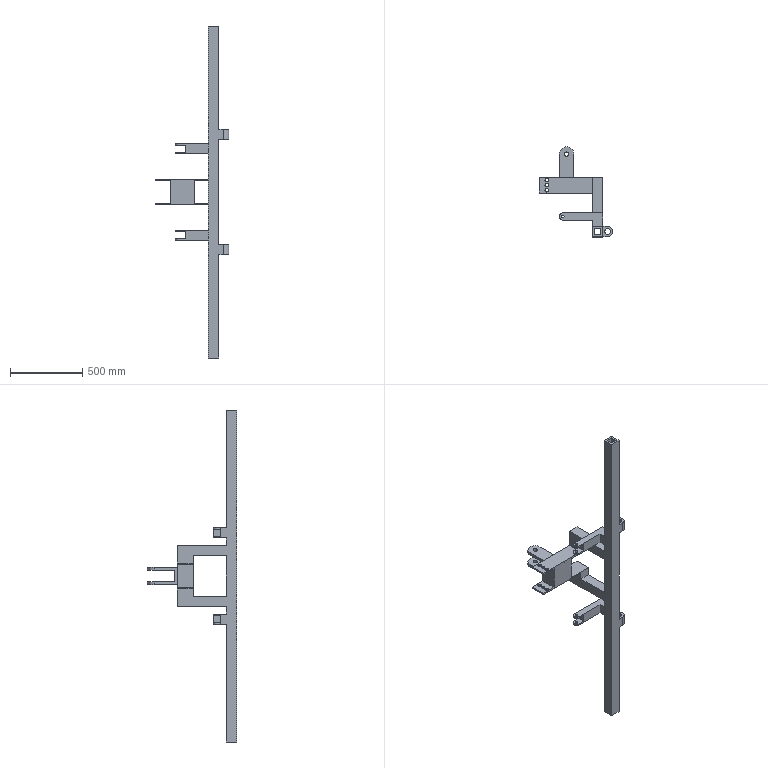Part | SolidWorks | 1 solid | 101 faces | box 510 x 622 x 2300 mm | volume 17041991 mm3 | plane 61 | cylinder 40 | commonest cylinder face diameters 25 x12 20 x8 50 x6 30 x4 40 x4 72 x4